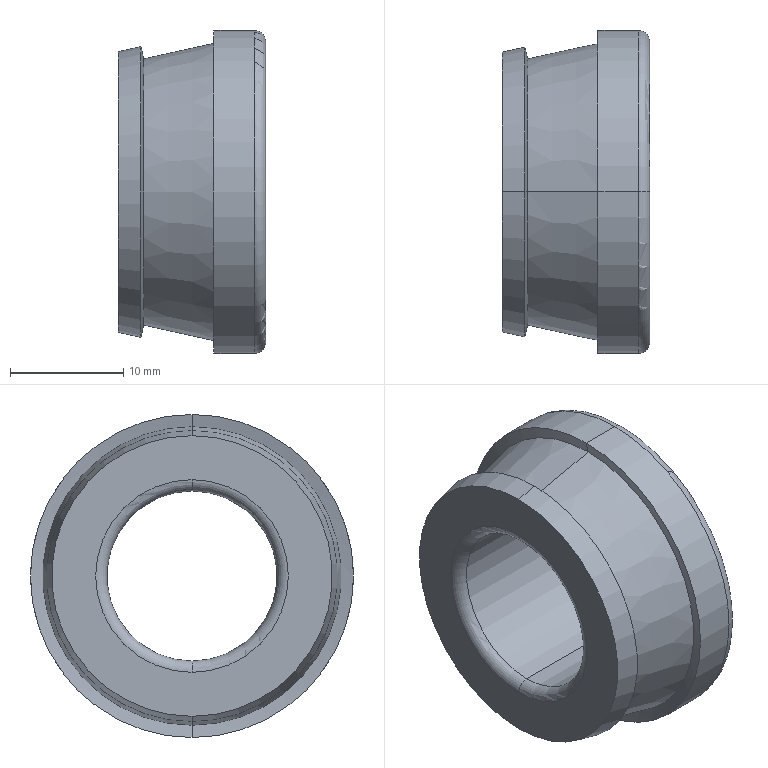Part | NX | features BREP 1 | 1 solid | 20 faces | box 13 x 28.5 x 28.5 mm | volume 4682 mm3 | cone 8 | torus 6 | cylinder 4 | plane 2 | commonest cylinder face diameters 15 x2 28.5 x2
STEP:
#1=CARTESIAN_POINT('',(12.,0.,-7.5));
#2=VERTEX_POINT('',#1);
#3=CARTESIAN_POINT('',(12.,0.,7.5));
#4=VERTEX_POINT('',#3);
#5=CARTESIAN_POINT('',(12.,0.,0.));
#6=DIRECTION('',(-1.,0.,0.));
#7=DIRECTION('',(0.,0.,-1.));
#8=AXIS2_PLACEMENT_3D('',#5,#6,#7);
#9=CIRCLE('',#8,7.5);
#10=EDGE_CURVE('',#2,#4,#9,.T.);
#11=ORIENTED_EDGE('',*,*,#10,.T.);
#12=CARTESIAN_POINT('',(13.,0.,8.5));
#13=VERTEX_POINT('',#12);
#14=CARTESIAN_POINT('',(12.,0.,8.5));
#15=DIRECTION('',(0.,1.,0.));
#16=DIRECTION('',(1.,0.,0.));
#17=AXIS2_PLACEMENT_3D('',#14,#15,#16);
#18=CIRCLE('',#17,1.);
#19=EDGE_CURVE('',#4,#13,#18,.F.);
#20=ORIENTED_EDGE('',*,*,#19,.T.);
#21=CARTESIAN_POINT('',(13.,0.,-8.5));
#22=VERTEX_POINT('',#21);
#23=CARTESIAN_POINT('',(13.,0.,0.));
#24=DIRECTION('',(-1.,0.,0.));
#25=DIRECTION('',(0.,0.,-1.));
#26=AXIS2_PLACEMENT_3D('',#23,#24,#25);
#27=CIRCLE('',#26,8.5);
#28=EDGE_CURVE('',#22,#13,#27,.T.);
#29=ORIENTED_EDGE('',*,*,#28,.F.);
#30=CARTESIAN_POINT('',(12.,0.,-8.5));
#31=DIRECTION('',(0.,-1.,0.));
#32=DIRECTION('',(1.,0.,0.));
#33=AXIS2_PLACEMENT_3D('',#30,#31,#32);
#34=CIRCLE('',#33,1.);
#35=EDGE_CURVE('',#2,#22,#34,.F.);
#36=ORIENTED_EDGE('',*,*,#35,.F.);
#37=EDGE_LOOP('',(#11,#20,#29,#36));
#38=FACE_BOUND('',#37,.T.);
#39=CARTESIAN_POINT('',(12.,0.,0.));
#40=DIRECTION('',(-1.,0.,0.));
#41=DIRECTION('',(0.,0.,1.));
#42=AXIS2_PLACEMENT_3D('',#39,#40,#41);
#43=TOROIDAL_SURFACE('',#42,8.5,1.);
#44=ADVANCED_FACE('',(#38),#43,.T.);
#45=ORIENTED_EDGE('',*,*,#35,.T.);
#46=CARTESIAN_POINT('',(13.,0.,0.));
#47=DIRECTION('',(-1.,0.,0.));
#48=DIRECTION('',(0.,0.,1.));
#49=AXIS2_PLACEMENT_3D('',#46,#47,#48);
#50=CIRCLE('',#49,8.5);
#51=EDGE_CURVE('',#13,#22,#50,.T.);
#52=ORIENTED_EDGE('',*,*,#51,.F.);
#53=ORIENTED_EDGE('',*,*,#19,.F.);
#54=CARTESIAN_POINT('',(12.,0.,0.));
#55=DIRECTION('',(-1.,0.,0.));
#56=DIRECTION('',(0.,0.,1.));
#57=AXIS2_PLACEMENT_3D('',#54,#55,#56);
#58=CIRCLE('',#57,7.5);
#59=EDGE_CURVE('',#4,#2,#58,.T.);
#60=ORIENTED_EDGE('',*,*,#59,.T.);
#61=EDGE_LOOP('',(#45,#52,#53,#60));
#62=FACE_BOUND('',#61,.T.);
#63=CARTESIAN_POINT('',(12.,0.,0.));
#64=DIRECTION('',(-1.,0.,0.));
#65=DIRECTION('',(0.,0.,1.));
#66=AXIS2_PLACEMENT_3D('',#63,#64,#65);
#67=TOROIDAL_SURFACE('',#66,8.5,1.);
#68=ADVANCED_FACE('',(#62),#67,.T.);
#69=ORIENTED_EDGE('',*,*,#59,.F.);
#70=CARTESIAN_POINT('',(1.,0.,7.5));
#71=VERTEX_POINT('',#70);
#72=CARTESIAN_POINT('',(1.,0.,7.5));
#73=DIRECTION('',(1.,0.,0.));
#74=VECTOR('',#73,1000.);
#75=LINE('',#72,#74);
#76=EDGE_CURVE('',#4,#71,#75,.F.);
#77=ORIENTED_EDGE('',*,*,#76,.T.);
#78=CARTESIAN_POINT('',(1.,0.,-7.5));
#79=VERTEX_POINT('',#78);
#80=CARTESIAN_POINT('',(1.,0.,0.));
#81=DIRECTION('',(1.,0.,0.));
#82=DIRECTION('',(0.,0.,-1.));
#83=AXIS2_PLACEMENT_3D('',#80,#81,#82);
#84=CIRCLE('',#83,7.5);
#85=EDGE_CURVE('',#79,#71,#84,.T.);
#86=ORIENTED_EDGE('',*,*,#85,.F.);
#87=CARTESIAN_POINT('',(1.,0.,-7.5));
#88=DIRECTION('',(1.,0.,0.));
#89=VECTOR('',#88,1000.);
#90=LINE('',#87,#89);
#91=EDGE_CURVE('',#2,#79,#90,.F.);
#92=ORIENTED_EDGE('',*,*,#91,.F.);
#93=EDGE_LOOP('',(#69,#77,#86,#92));
#94=FACE_BOUND('',#93,.T.);
#95=CARTESIAN_POINT('',(0.,0.,0.));
#96=DIRECTION('',(-1.,0.,0.));
#97=DIRECTION('',(0.,0.,1.));
#98=AXIS2_PLACEMENT_3D('',#95,#96,#97);
#99=CYLINDRICAL_SURFACE('',#98,7.5);
#100=ADVANCED_FACE('',(#94),#99,.F.);
#101=ORIENTED_EDGE('',*,*,#91,.T.);
#102=CARTESIAN_POINT('',(1.,0.,0.));
#103=DIRECTION('',(1.,0.,0.));
#104=DIRECTION('',(0.,0.,1.));
#105=AXIS2_PLACEMENT_3D('',#102,#103,#104);
#106=CIRCLE('',#105,7.5);
#107=EDGE_CURVE('',#71,#79,#106,.T.);
#108=ORIENTED_EDGE('',*,*,#107,.F.);
#109=ORIENTED_EDGE('',*,*,#76,.F.);
#110=ORIENTED_EDGE('',*,*,#10,.F.);
#111=EDGE_LOOP('',(#101,#108,#109,#110));
#112=FACE_BOUND('',#111,.T.);
#113=CARTESIAN_POINT('',(0.,0.,0.));
#114=DIRECTION('',(-1.,0.,0.));
#115=DIRECTION('',(0.,0.,1.));
#116=AXIS2_PLACEMENT_3D('',#113,#114,#115);
#117=CYLINDRICAL_SURFACE('',#116,7.5);
#118=ADVANCED_FACE('',(#112),#117,.F.);
#119=ORIENTED_EDGE('',*,*,#107,.T.);
#120=CARTESIAN_POINT('',(0.,0.,-8.5));
#121=VERTEX_POINT('',#120);
#122=CARTESIAN_POINT('',(1.,0.,-8.5));
#123=DIRECTION('',(0.,1.,0.));
#124=DIRECTION('',(-1.,0.,0.));
#125=AXIS2_PLACEMENT_3D('',#122,#123,#124);
#126=CIRCLE('',#125,1.);
#127=EDGE_CURVE('',#121,#79,#126,.T.);
#128=ORIENTED_EDGE('',*,*,#127,.F.);
#129=CARTESIAN_POINT('',(0.,0.,8.5));
#130=VERTEX_POINT('',#129);
#131=CARTESIAN_POINT('',(0.,0.,0.));
#132=DIRECTION('',(1.,0.,0.));
#133=DIRECTION('',(0.,0.,1.));
#134=AXIS2_PLACEMENT_3D('',#131,#132,#133);
#135=CIRCLE('',#134,8.5);
#136=EDGE_CURVE('',#130,#121,#135,.T.);
#137=ORIENTED_EDGE('',*,*,#136,.F.);
#138=CARTESIAN_POINT('',(1.,0.,8.5));
#139=DIRECTION('',(0.,-1.,0.));
#140=DIRECTION('',(-1.,0.,0.));
#141=AXIS2_PLACEMENT_3D('',#138,#139,#140);
#142=CIRCLE('',#141,1.);
#143=EDGE_CURVE('',#130,#71,#142,.T.);
#144=ORIENTED_EDGE('',*,*,#143,.T.);
#145=EDGE_LOOP('',(#119,#128,#137,#144));
#146=FACE_BOUND('',#145,.T.);
#147=CARTESIAN_POINT('',(1.,0.,0.));
#148=DIRECTION('',(1.,0.,0.));
#149=DIRECTION('',(0.,0.,-1.));
#150=AXIS2_PLACEMENT_3D('',#147,#148,#149);
#151=TOROIDAL_SURFACE('',#150,8.5,1.);
#152=ADVANCED_FACE('',(#146),#151,.T.);
#153=ORIENTED_EDGE('',*,*,#143,.F.);
#154=CARTESIAN_POINT('',(0.,0.,0.));
#155=DIRECTION('',(1.,0.,0.));
#156=DIRECTION('',(0.,0.,-1.));
#157=AXIS2_PLACEMENT_3D('',#154,#155,#156);
#158=CIRCLE('',#157,8.5);
#159=EDGE_CURVE('',#121,#130,#158,.T.);
#160=ORIENTED_EDGE('',*,*,#159,.F.);
#161=ORIENTED_EDGE('',*,*,#127,.T.);
#162=ORIENTED_EDGE('',*,*,#85,.T.);
#163=EDGE_LOOP('',(#153,#160,#161,#162));
#164=FACE_BOUND('',#163,.T.);
#165=CARTESIAN_POINT('',(1.,0.,0.));
#166=DIRECTION('',(1.,0.,0.));
#167=DIRECTION('',(0.,0.,-1.));
#168=AXIS2_PLACEMENT_3D('',#165,#166,#167);
#169=TOROIDAL_SURFACE('',#168,8.5,1.);
#170=ADVANCED_FACE('',(#164),#169,.T.);
#171=CARTESIAN_POINT('',(0.,0.,12.38));
#172=VERTEX_POINT('',#171);
#173=CARTESIAN_POINT('',(0.,0.,-12.38));
#174=VERTEX_POINT('',#173);
#175=CARTESIAN_POINT('',(0.,0.,0.));
#176=DIRECTION('',(-1.,0.,0.));
#177=DIRECTION('',(0.,0.,1.));
#178=AXIS2_PLACEMENT_3D('',#175,#176,#177);
#179=CIRCLE('',#178,12.38);
#180=EDGE_CURVE('',#172,#174,#179,.T.);
#181=ORIENTED_EDGE('',*,*,#180,.T.);
#182=CARTESIAN_POINT('',(0.,0.,0.));
#183=DIRECTION('',(-1.,0.,0.));
#184=DIRECTION('',(0.,0.,-1.));
#185=AXIS2_PLACEMENT_3D('',#182,#183,#184);
#186=CIRCLE('',#185,12.38);
#187=EDGE_CURVE('',#174,#172,#186,.T.);
#188=ORIENTED_EDGE('',*,*,#187,.T.);
#189=EDGE_LOOP('',(#181,#188));
#190=FACE_BOUND('',#189,.T.);
#191=ORIENTED_EDGE('',*,*,#136,.T.);
#192=ORIENTED_EDGE('',*,*,#159,.T.);
#193=EDGE_LOOP('',(#191,#192));
#194=FACE_BOUND('',#193,.T.);
#195=CARTESIAN_POINT('',(0.,7.5,0.));
#196=DIRECTION('',(1.,0.,0.));
#197=DIRECTION('',(0.,1.,0.));
#198=AXIS2_PLACEMENT_3D('',#195,#196,#197);
#199=PLANE('',#198);
#200=ADVANCED_FACE('',(#190,#194),#199,.F.);
#201=ORIENTED_EDGE('',*,*,#187,.F.);
#202=CARTESIAN_POINT('',(1.992,0.,-12.821));
#203=VERTEX_POINT('',#202);
#204=CARTESIAN_POINT('',(1.992,0.,-12.821));
#205=DIRECTION('',(-0.9763,0.,0.2164));
#206=VECTOR('',#205,1000.);
#207=LINE('',#204,#206);
#208=EDGE_CURVE('',#203,#174,#207,.T.);
#209=ORIENTED_EDGE('',*,*,#208,.F.);
#210=CARTESIAN_POINT('',(1.992,0.,12.821));
#211=VERTEX_POINT('',#210);
#212=CARTESIAN_POINT('',(1.992,0.,0.));
#213=DIRECTION('',(1.,0.,0.));
#214=DIRECTION('',(0.,0.,1.));
#215=AXIS2_PLACEMENT_3D('',#212,#213,#214);
#216=CIRCLE('',#215,12.821);
#217=EDGE_CURVE('',#211,#203,#216,.T.);
#218=ORIENTED_EDGE('',*,*,#217,.F.);
#219=CARTESIAN_POINT('',(1.992,0.,12.821));
#220=DIRECTION('',(-0.9763,0.,-0.2164));
#221=VECTOR('',#220,1000.);
#222=LINE('',#219,#221);
#223=EDGE_CURVE('',#211,#172,#222,.T.);
#224=ORIENTED_EDGE('',*,*,#223,.T.);
#225=EDGE_LOOP('',(#201,#209,#218,#224));
#226=FACE_BOUND('',#225,.T.);
#227=CARTESIAN_POINT('',(0.9958,0.,0.));
#228=DIRECTION('',(1.,0.,0.));
#229=DIRECTION('',(0.,0.,-1.));
#230=AXIS2_PLACEMENT_3D('',#227,#228,#229);
#231=CONICAL_SURFACE('',#230,12.601,0.2182);
#232=ADVANCED_FACE('',(#226),#231,.T.);
#233=ORIENTED_EDGE('',*,*,#223,.F.);
#234=CARTESIAN_POINT('',(1.992,0.,0.));
#235=DIRECTION('',(1.,0.,0.));
#236=DIRECTION('',(0.,0.,-1.));
#237=AXIS2_PLACEMENT_3D('',#234,#235,#236);
#238=CIRCLE('',#237,12.821);
#239=EDGE_CURVE('',#203,#211,#238,.T.);
#240=ORIENTED_EDGE('',*,*,#239,.F.);
#241=ORIENTED_EDGE('',*,*,#208,.T.);
#242=ORIENTED_EDGE('',*,*,#180,.F.);
#243=EDGE_LOOP('',(#233,#240,#241,#242));
#244=FACE_BOUND('',#243,.T.);
#245=CARTESIAN_POINT('',(0.9958,0.,0.));
#246=DIRECTION('',(1.,0.,0.));
#247=DIRECTION('',(0.,0.,-1.));
#248=AXIS2_PLACEMENT_3D('',#245,#246,#247);
#249=CONICAL_SURFACE('',#248,12.601,0.2182);
#250=ADVANCED_FACE('',(#244),#249,.T.);
#251=CARTESIAN_POINT('',(2.232,0.,-11.736));
#252=VERTEX_POINT('',#251);
#253=CARTESIAN_POINT('',(1.992,0.,-12.821));
#254=DIRECTION('',(0.2164,0.,0.9763));
#255=VECTOR('',#254,1000.);
#256=LINE('',#253,#255);
#257=EDGE_CURVE('',#203,#252,#256,.T.);
#258=ORIENTED_EDGE('',*,*,#257,.F.);
#259=ORIENTED_EDGE('',*,*,#239,.T.);
#260=CARTESIAN_POINT('',(2.232,0.,11.736));
#261=VERTEX_POINT('',#260);
#262=CARTESIAN_POINT('',(1.992,0.,12.821));
#263=DIRECTION('',(0.2164,0.,-0.9763));
#264=VECTOR('',#263,1000.);
#265=LINE('',#262,#264);
#266=EDGE_CURVE('',#211,#261,#265,.T.);
#267=ORIENTED_EDGE('',*,*,#266,.T.);
#268=CARTESIAN_POINT('',(2.232,0.,0.));
#269=DIRECTION('',(1.,0.,0.));
#270=DIRECTION('',(0.,0.,-1.));
#271=AXIS2_PLACEMENT_3D('',#268,#269,#270);
#272=CIRCLE('',#271,11.736);
#273=EDGE_CURVE('',#252,#261,#272,.T.);
#274=ORIENTED_EDGE('',*,*,#273,.F.);
#275=EDGE_LOOP('',(#258,#259,#267,#274));
#276=FACE_BOUND('',#275,.T.);
#277=CARTESIAN_POINT('',(2.112,0.,0.));
#278=DIRECTION('',(-1.,0.,0.));
#279=DIRECTION('',(0.,0.,1.));
#280=AXIS2_PLACEMENT_3D('',#277,#278,#279);
#281=CONICAL_SURFACE('',#280,12.279,1.353);
#282=ADVANCED_FACE('',(#276),#281,.T.);
#283=CARTESIAN_POINT('',(8.676,0.,13.165));
#284=VERTEX_POINT('',#283);
#285=CARTESIAN_POINT('',(8.676,0.,13.165));
#286=DIRECTION('',(-0.9763,0.,-0.2164));
#287=VECTOR('',#286,1000.);
#288=LINE('',#285,#287);
#289=EDGE_CURVE('',#261,#284,#288,.F.);
#290=ORIENTED_EDGE('',*,*,#289,.T.);
#291=CARTESIAN_POINT('',(8.676,0.,-13.165));
#292=VERTEX_POINT('',#291);
#293=CARTESIAN_POINT('',(8.676,0.,0.));
#294=DIRECTION('',(1.,0.,0.));
#295=DIRECTION('',(0.,0.,-1.));
#296=AXIS2_PLACEMENT_3D('',#293,#294,#295);
#297=CIRCLE('',#296,13.165);
#298=EDGE_CURVE('',#292,#284,#297,.T.);
#299=ORIENTED_EDGE('',*,*,#298,.F.);
#300=CARTESIAN_POINT('',(8.676,0.,-13.165));
#301=DIRECTION('',(-0.9763,0.,0.2164));
#302=VECTOR('',#301,1000.);
#303=LINE('',#300,#302);
#304=EDGE_CURVE('',#252,#292,#303,.F.);
#305=ORIENTED_EDGE('',*,*,#304,.F.);
#306=ORIENTED_EDGE('',*,*,#273,.T.);
#307=EDGE_LOOP('',(#290,#299,#305,#306));
#308=FACE_BOUND('',#307,.T.);
#309=CARTESIAN_POINT('',(5.454,0.,0.));
#310=DIRECTION('',(1.,0.,0.));
#311=DIRECTION('',(0.,0.,-1.));
#312=AXIS2_PLACEMENT_3D('',#309,#310,#311);
#313=CONICAL_SURFACE('',#312,12.45,0.2182);
#314=ADVANCED_FACE('',(#308),#313,.T.);
#315=CARTESIAN_POINT('',(2.232,0.,0.));
#316=DIRECTION('',(1.,0.,0.));
#317=DIRECTION('',(0.,0.,1.));
#318=AXIS2_PLACEMENT_3D('',#315,#316,#317);
#319=CIRCLE('',#318,11.736);
#320=EDGE_CURVE('',#261,#252,#319,.T.);
#321=ORIENTED_EDGE('',*,*,#320,.T.);
#322=ORIENTED_EDGE('',*,*,#304,.T.);
#323=CARTESIAN_POINT('',(8.676,0.,0.));
#324=DIRECTION('',(1.,0.,0.));
#325=DIRECTION('',(0.,0.,1.));
#326=AXIS2_PLACEMENT_3D('',#323,#324,#325);
#327=CIRCLE('',#326,13.165);
#328=EDGE_CURVE('',#284,#292,#327,.T.);
#329=ORIENTED_EDGE('',*,*,#328,.F.);
#330=ORIENTED_EDGE('',*,*,#289,.F.);
#331=EDGE_LOOP('',(#321,#322,#329,#330));
#332=FACE_BOUND('',#331,.T.);
#333=CARTESIAN_POINT('',(5.454,0.,0.));
#334=DIRECTION('',(1.,0.,0.));
#335=DIRECTION('',(0.,0.,-1.));
#336=AXIS2_PLACEMENT_3D('',#333,#334,#335);
#337=CONICAL_SURFACE('',#336,12.45,0.2182);
#338=ADVANCED_FACE('',(#332),#337,.T.);
#339=CARTESIAN_POINT('',(8.435,0.,-14.25));
#340=VERTEX_POINT('',#339);
#341=CARTESIAN_POINT('',(8.435,0.,-14.25));
#342=DIRECTION('',(0.2164,0.,0.9763));
#343=VECTOR('',#342,1000.);
#344=LINE('',#341,#343);
#345=EDGE_CURVE('',#340,#292,#344,.T.);
#346=ORIENTED_EDGE('',*,*,#345,.F.);
#347=CARTESIAN_POINT('',(8.435,0.,14.25));
#348=VERTEX_POINT('',#347);
#349=CARTESIAN_POINT('',(8.435,0.,0.));
#350=DIRECTION('',(-1.,0.,0.));
#351=DIRECTION('',(0.,0.,-1.));
#352=AXIS2_PLACEMENT_3D('',#349,#350,#351);
#353=CIRCLE('',#352,14.25);
#354=EDGE_CURVE('',#340,#348,#353,.T.);
#355=ORIENTED_EDGE('',*,*,#354,.T.);
#356=CARTESIAN_POINT('',(8.435,0.,14.25));
#357=DIRECTION('',(0.2164,0.,-0.9763));
#358=VECTOR('',#357,1000.);
#359=LINE('',#356,#358);
#360=EDGE_CURVE('',#348,#284,#359,.T.);
#361=ORIENTED_EDGE('',*,*,#360,.T.);
#362=ORIENTED_EDGE('',*,*,#328,.T.);
#363=EDGE_LOOP('',(#346,#355,#361,#362));
#364=FACE_BOUND('',#363,.T.);
#365=CARTESIAN_POINT('',(8.556,0.,0.));
#366=DIRECTION('',(-1.,0.,0.));
#367=DIRECTION('',(0.,0.,1.));
#368=AXIS2_PLACEMENT_3D('',#365,#366,#367);
#369=CONICAL_SURFACE('',#368,13.707,1.353);
#370=ADVANCED_FACE('',(#364),#369,.F.);
#371=ORIENTED_EDGE('',*,*,#298,.T.);
#372=ORIENTED_EDGE('',*,*,#360,.F.);
#373=CARTESIAN_POINT('',(8.435,0.,0.));
#374=DIRECTION('',(-1.,0.,0.));
#375=DIRECTION('',(0.,0.,1.));
#376=AXIS2_PLACEMENT_3D('',#373,#374,#375);
#377=CIRCLE('',#376,14.25);
#378=EDGE_CURVE('',#348,#340,#377,.T.);
#379=ORIENTED_EDGE('',*,*,#378,.T.);
#380=ORIENTED_EDGE('',*,*,#345,.T.);
#381=EDGE_LOOP('',(#371,#372,#379,#380));
#382=FACE_BOUND('',#381,.T.);
#383=CARTESIAN_POINT('',(8.556,0.,0.));
#384=DIRECTION('',(-1.,0.,0.));
#385=DIRECTION('',(0.,0.,1.));
#386=AXIS2_PLACEMENT_3D('',#383,#384,#385);
#387=CONICAL_SURFACE('',#386,13.707,1.353);
#388=ADVANCED_FACE('',(#382),#387,.F.);
#389=CARTESIAN_POINT('',(12.,0.,-14.25));
#390=VERTEX_POINT('',#389);
#391=CARTESIAN_POINT('',(8.435,0.,-14.25));
#392=DIRECTION('',(1.,0.,0.));
#393=VECTOR('',#392,1000.);
#394=LINE('',#391,#393);
#395=EDGE_CURVE('',#340,#390,#394,.T.);
#396=ORIENTED_EDGE('',*,*,#395,.F.);
#397=ORIENTED_EDGE('',*,*,#378,.F.);
#398=CARTESIAN_POINT('',(12.,0.,14.25));
#399=VERTEX_POINT('',#398);
#400=CARTESIAN_POINT('',(8.435,0.,14.25));
#401=DIRECTION('',(1.,0.,0.));
#402=VECTOR('',#401,1000.);
#403=LINE('',#400,#402);
#404=EDGE_CURVE('',#348,#399,#403,.T.);
#405=ORIENTED_EDGE('',*,*,#404,.T.);
#406=CARTESIAN_POINT('',(12.,0.,0.));
#407=DIRECTION('',(1.,0.,0.));
#408=DIRECTION('',(0.,0.,-1.));
#409=AXIS2_PLACEMENT_3D('',#406,#407,#408);
#410=CIRCLE('',#409,14.25);
#411=EDGE_CURVE('',#390,#399,#410,.T.);
#412=ORIENTED_EDGE('',*,*,#411,.F.);
#413=EDGE_LOOP('',(#396,#397,#405,#412));
#414=FACE_BOUND('',#413,.T.);
#415=CARTESIAN_POINT('',(0.,0.,0.));
#416=DIRECTION('',(-1.,0.,0.));
#417=DIRECTION('',(0.,0.,1.));
#418=AXIS2_PLACEMENT_3D('',#415,#416,#417);
#419=CYLINDRICAL_SURFACE('',#418,14.25);
#420=ADVANCED_FACE('',(#414),#419,.T.);
#421=CARTESIAN_POINT('',(13.,0.,-13.25));
#422=VERTEX_POINT('',#421);
#423=CARTESIAN_POINT('',(12.,0.,-13.25));
#424=DIRECTION('',(0.,-1.,0.));
#425=DIRECTION('',(0.,0.,-1.));
#426=AXIS2_PLACEMENT_3D('',#423,#424,#425);
#427=CIRCLE('',#426,1.);
#428=EDGE_CURVE('',#390,#422,#427,.T.);
#429=ORIENTED_EDGE('',*,*,#428,.F.);
#430=ORIENTED_EDGE('',*,*,#411,.T.);
#431=CARTESIAN_POINT('',(13.,0.,13.25));
#432=VERTEX_POINT('',#431);
#433=CARTESIAN_POINT('',(12.,0.,13.25));
#434=DIRECTION('',(0.,1.,0.));
#435=DIRECTION('',(0.,0.,1.));
#436=AXIS2_PLACEMENT_3D('',#433,#434,#435);
#437=CIRCLE('',#436,1.);
#438=EDGE_CURVE('',#399,#432,#437,.T.);
#439=ORIENTED_EDGE('',*,*,#438,.T.);
#440=CARTESIAN_POINT('',(13.,0.,0.));
#441=DIRECTION('',(1.,0.,0.));
#442=DIRECTION('',(0.,0.,-1.));
#443=AXIS2_PLACEMENT_3D('',#440,#441,#442);
#444=CIRCLE('',#443,13.25);
#445=EDGE_CURVE('',#422,#432,#444,.T.);
#446=ORIENTED_EDGE('',*,*,#445,.F.);
#447=EDGE_LOOP('',(#429,#430,#439,#446));
#448=FACE_BOUND('',#447,.T.);
#449=CARTESIAN_POINT('',(12.,0.,0.));
#450=DIRECTION('',(-1.,0.,0.));
#451=DIRECTION('',(0.,0.,1.));
#452=AXIS2_PLACEMENT_3D('',#449,#450,#451);
#453=TOROIDAL_SURFACE('',#452,13.25,1.);
#454=ADVANCED_FACE('',(#448),#453,.T.);
#455=ORIENTED_EDGE('',*,*,#445,.T.);
#456=CARTESIAN_POINT('',(13.,0.,0.));
#457=DIRECTION('',(1.,0.,0.));
#458=DIRECTION('',(0.,0.,1.));
#459=AXIS2_PLACEMENT_3D('',#456,#457,#458);
#460=CIRCLE('',#459,13.25);
#461=EDGE_CURVE('',#432,#422,#460,.T.);
#462=ORIENTED_EDGE('',*,*,#461,.T.);
#463=EDGE_LOOP('',(#455,#462));
#464=FACE_BOUND('',#463,.T.);
#465=ORIENTED_EDGE('',*,*,#28,.T.);
#466=ORIENTED_EDGE('',*,*,#51,.T.);
#467=EDGE_LOOP('',(#465,#466));
#468=FACE_BOUND('',#467,.T.);
#469=CARTESIAN_POINT('',(13.,14.25,0.));
#470=DIRECTION('',(-1.,0.,0.));
#471=DIRECTION('',(0.,0.,1.));
#472=AXIS2_PLACEMENT_3D('',#469,#470,#471);
#473=PLANE('',#472);
#474=ADVANCED_FACE('',(#464,#468),#473,.F.);
#475=ORIENTED_EDGE('',*,*,#461,.F.);
#476=ORIENTED_EDGE('',*,*,#438,.F.);
#477=CARTESIAN_POINT('',(12.,0.,0.));
#478=DIRECTION('',(1.,0.,0.));
#479=DIRECTION('',(0.,0.,1.));
#480=AXIS2_PLACEMENT_3D('',#477,#478,#479);
#481=CIRCLE('',#480,14.25);
#482=EDGE_CURVE('',#399,#390,#481,.T.);
#483=ORIENTED_EDGE('',*,*,#482,.T.);
#484=ORIENTED_EDGE('',*,*,#428,.T.);
#485=EDGE_LOOP('',(#475,#476,#483,#484));
#486=FACE_BOUND('',#485,.T.);
#487=CARTESIAN_POINT('',(12.,0.,0.));
#488=DIRECTION('',(-1.,0.,0.));
#489=DIRECTION('',(0.,0.,1.));
#490=AXIS2_PLACEMENT_3D('',#487,#488,#489);
#491=TOROIDAL_SURFACE('',#490,13.25,1.);
#492=ADVANCED_FACE('',(#486),#491,.T.);
#493=ORIENTED_EDGE('',*,*,#482,.F.);
#494=ORIENTED_EDGE('',*,*,#404,.F.);
#495=ORIENTED_EDGE('',*,*,#354,.F.);
#496=ORIENTED_EDGE('',*,*,#395,.T.);
#497=EDGE_LOOP('',(#493,#494,#495,#496));
#498=FACE_BOUND('',#497,.T.);
#499=CARTESIAN_POINT('',(0.,0.,0.));
#500=DIRECTION('',(-1.,0.,0.));
#501=DIRECTION('',(0.,0.,1.));
#502=AXIS2_PLACEMENT_3D('',#499,#500,#501);
#503=CYLINDRICAL_SURFACE('',#502,14.25);
#504=ADVANCED_FACE('',(#498),#503,.T.);
#505=ORIENTED_EDGE('',*,*,#320,.F.);
#506=ORIENTED_EDGE('',*,*,#266,.F.);
#507=ORIENTED_EDGE('',*,*,#217,.T.);
#508=ORIENTED_EDGE('',*,*,#257,.T.);
#509=EDGE_LOOP('',(#505,#506,#507,#508));
#510=FACE_BOUND('',#509,.T.);
#511=CARTESIAN_POINT('',(2.112,0.,0.));
#512=DIRECTION('',(-1.,0.,0.));
#513=DIRECTION('',(0.,0.,1.));
#514=AXIS2_PLACEMENT_3D('',#511,#512,#513);
#515=CONICAL_SURFACE('',#514,12.279,1.353);
#516=ADVANCED_FACE('',(#510),#515,.T.);
#517=CLOSED_SHELL('',(#44,#68,#100,#118,#152,#170,#200,#232,#250,#282,#314,#338,#370,#388,#420,#454,#474,#492,#504,#516));
#518=MANIFOLD_SOLID_BREP('',#517);
#519=(LENGTH_UNIT()NAMED_UNIT(*)SI_UNIT(.MILLI.,.METRE.));
#520=UNCERTAINTY_MEASURE_WITH_UNIT(LENGTH_MEASURE(0.00001),#519,'','');
#521=(NAMED_UNIT(*)PLANE_ANGLE_UNIT()SI_UNIT($,.RADIAN.));
#522=(NAMED_UNIT(*)SI_UNIT($,.STERADIAN.)SOLID_ANGLE_UNIT());
#523=(GEOMETRIC_REPRESENTATION_CONTEXT(3)GLOBAL_UNCERTAINTY_ASSIGNED_CONTEXT((#520))GLOBAL_UNIT_ASSIGNED_CONTEXT((#519,#521,#522))REPRESENTATION_CONTEXT('',''));
#524=ADVANCED_BREP_SHAPE_REPRESENTATION('',(#518),#523);